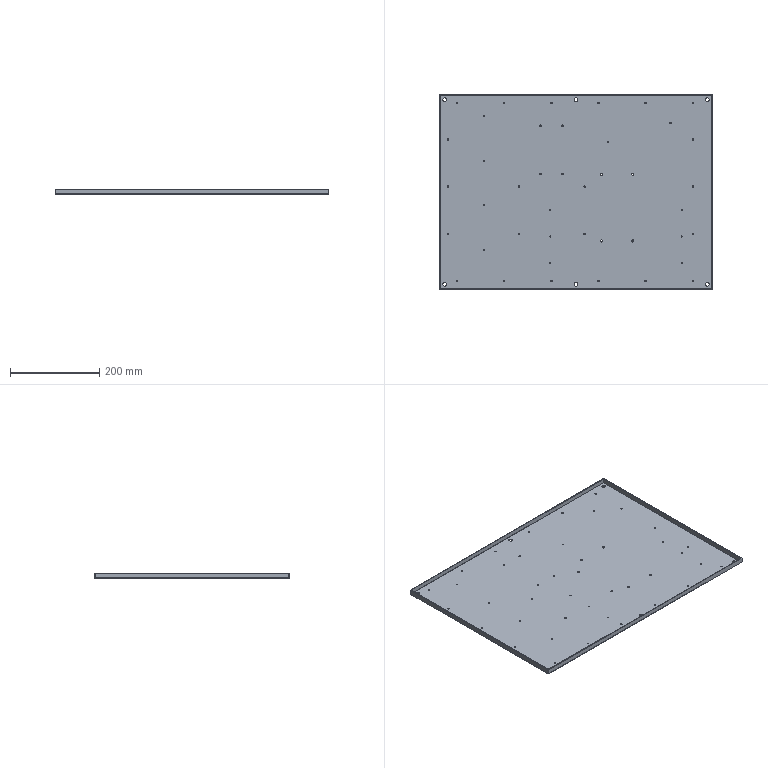Part | STEP file | CS-DS-002 | 1 solid | 142 faces | box 615 x 440 x 12 mm | volume 579701 mm3 | cylinder 104 | plane 30 | spline 8 | commonest cylinder face diameters 3.3 x56 2.5 x20 8 x12 4.8 x8 0.4 x4 4.4 x4